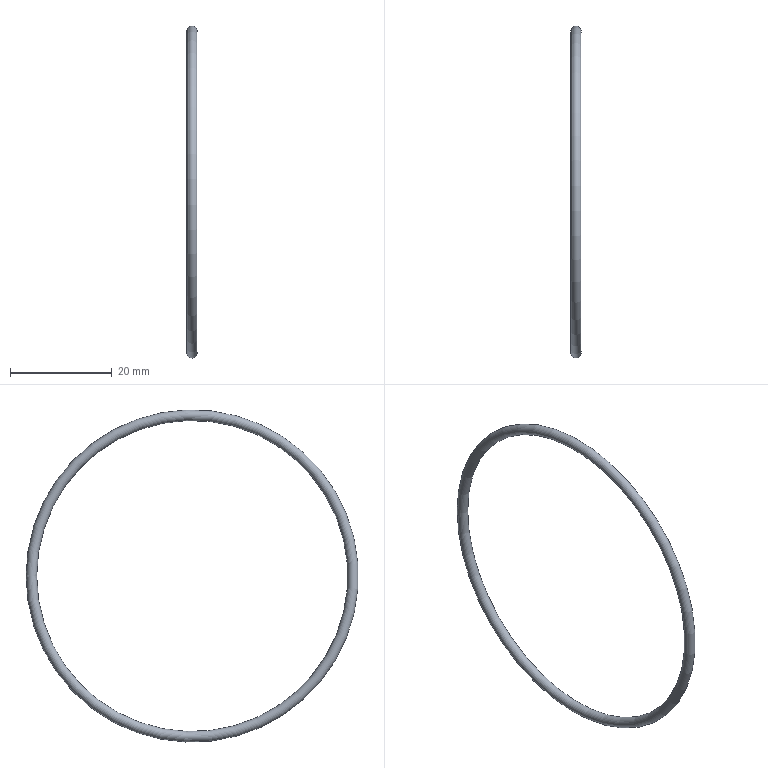Part | STEP file | Spring [2] | 1 solid | 2 faces | box 2.08 x 65.33 x 65.33 mm | volume 399.131 mm3 | torus 2
STEP:
#1=CARTESIAN_POINT('',(2.64,0.,0.));
#2=DIRECTION('',(1.,0.,0.));
#3=DIRECTION('',(0.,1.,0.));
#4=AXIS2_PLACEMENT_3D('',#1,#2,#3);
#5=TOROIDAL_SURFACE('',#4,31.625,1.04);
#6=ADVANCED_FACE('',(),#5,.T.);
#7=CLOSED_SHELL('',(#6));
#8=CARTESIAN_POINT('',(2.64,0.,0.));
#9=DIRECTION('',(1.,0.,0.));
#10=DIRECTION('',(0.,1.,0.));
#11=AXIS2_PLACEMENT_3D('',#8,#9,#10);
#12=TOROIDAL_SURFACE('',#11,31.625,0.665);
#13=ADVANCED_FACE('',(),#12,.F.);
#14=CLOSED_SHELL('',(#13));
#15=ORIENTED_CLOSED_SHELL('',*,#14,.T.);
#16=BREP_WITH_VOIDS('',#7,(#15));
#17=(LENGTH_UNIT()NAMED_UNIT(*)SI_UNIT(.MILLI.,.METRE.));
#18=UNCERTAINTY_MEASURE_WITH_UNIT(LENGTH_MEASURE(0.00001),#17,'','');
#19=(NAMED_UNIT(*)PLANE_ANGLE_UNIT()SI_UNIT($,.RADIAN.));
#20=(NAMED_UNIT(*)SI_UNIT($,.STERADIAN.)SOLID_ANGLE_UNIT());
#21=(GEOMETRIC_REPRESENTATION_CONTEXT(3)GLOBAL_UNCERTAINTY_ASSIGNED_CONTEXT((#18))GLOBAL_UNIT_ASSIGNED_CONTEXT((#17,#19,#20))REPRESENTATION_CONTEXT('',''));
#22=ADVANCED_BREP_SHAPE_REPRESENTATION('',(#16),#21);